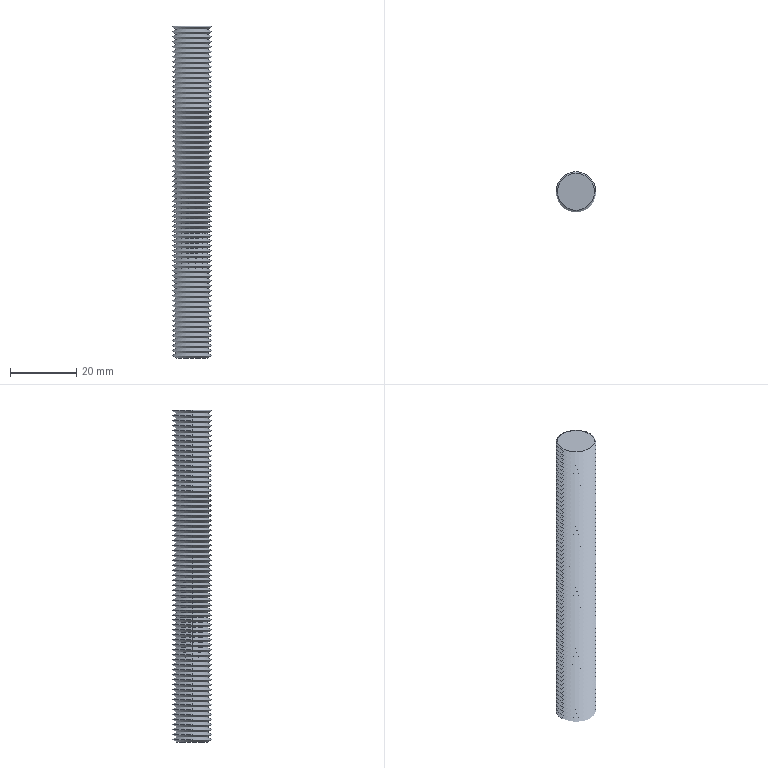Part | STEP file | GB/T15389-1994 screw rod M12×100 | 1 solid | 404 faces | box 12 x 12 x 100 mm | volume 9042 mm3 | cone 268 | cylinder 134 | plane 2 | commonest cylinder face diameters 12 x134